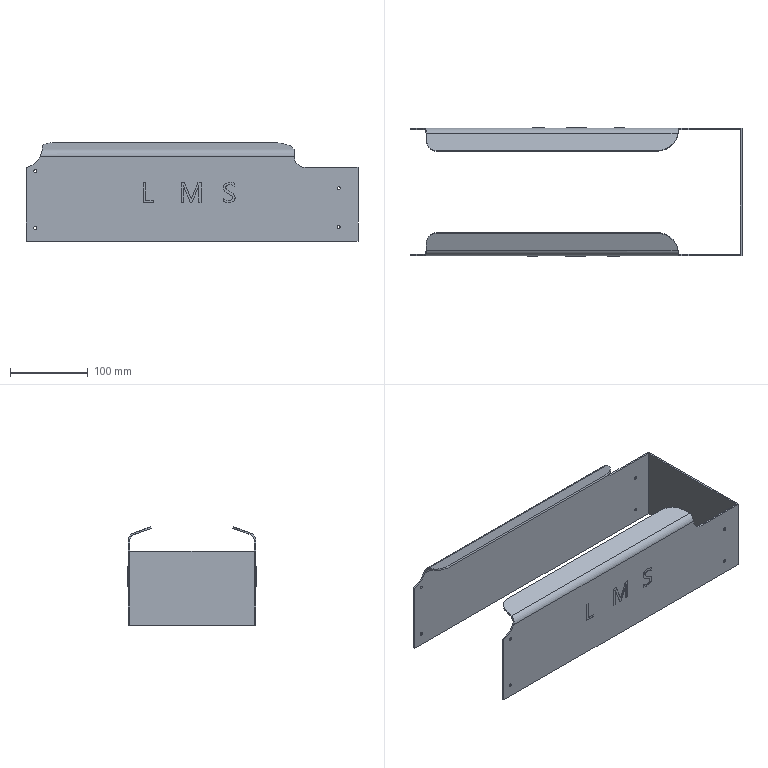Part | STEP file | 1-43.3 | 1 solid | 132 faces | box 427 x 165 x 126.605 mm | volume 256385 mm3 | plane 76 | spline 36 | cylinder 20 | commonest cylinder face diameters 4 x8 28 x4 16 x2 20 x2 52 x2 56 x2